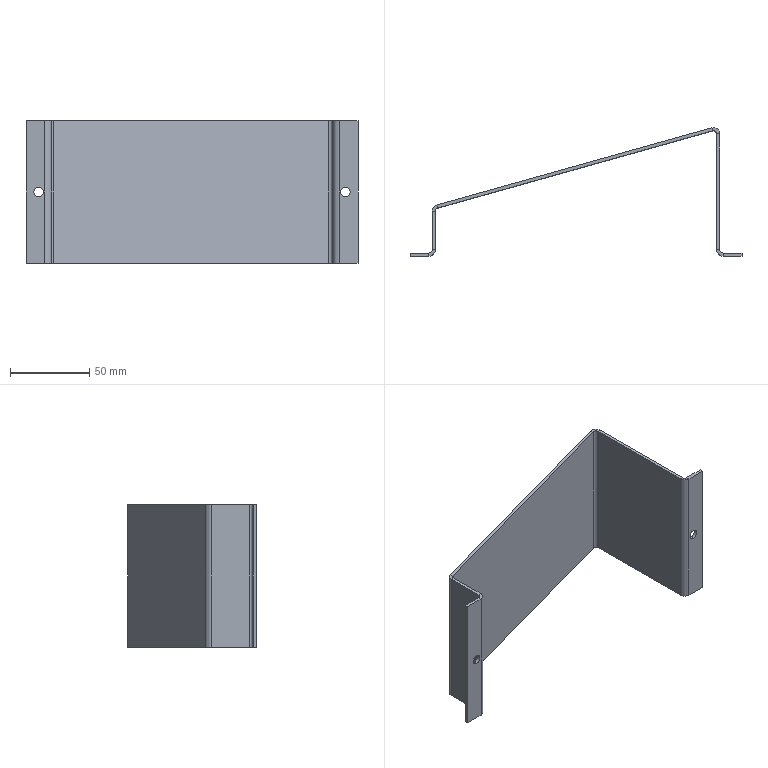Part | STEP file | 09-Protective cover | 1 solid | 42 faces | box 210 x 81.361 x 90 mm | volume 57744 mm3 | plane 30 | cylinder 12 | commonest cylinder face diameters 4 x4 6 x4 8 x4